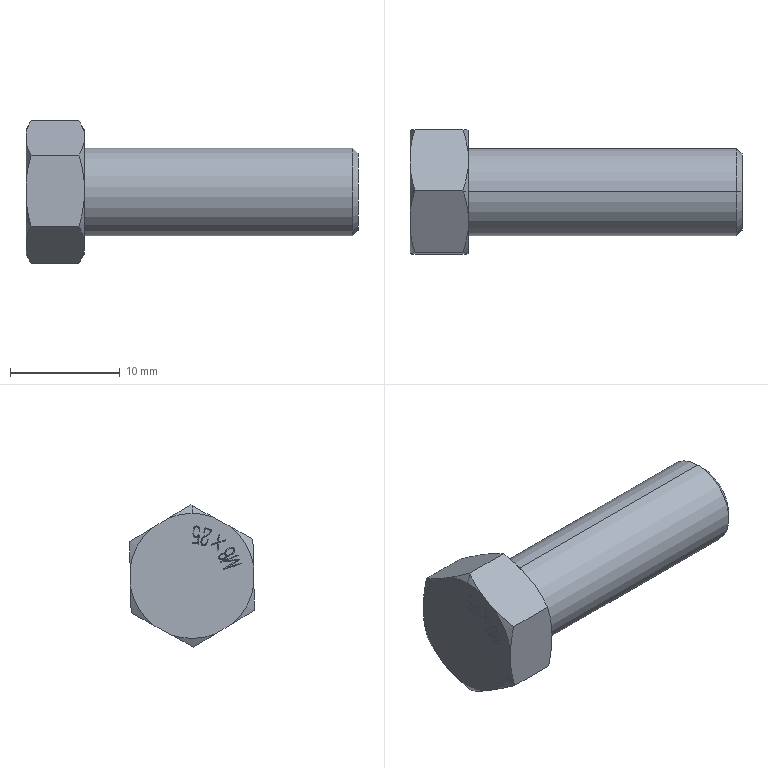Part | SolidWorks | features ICE 2, Chamfer 1, Extrusion 1, MirrorPattern 1, RevCut 1 | 1 solid | 143 faces | box 30.3 x 11.399 x 13 mm | volume 1833 mm3 | plane 75 | spline 50 | cone 16 | cylinder 2 | commonest cylinder face diameters 8 x2